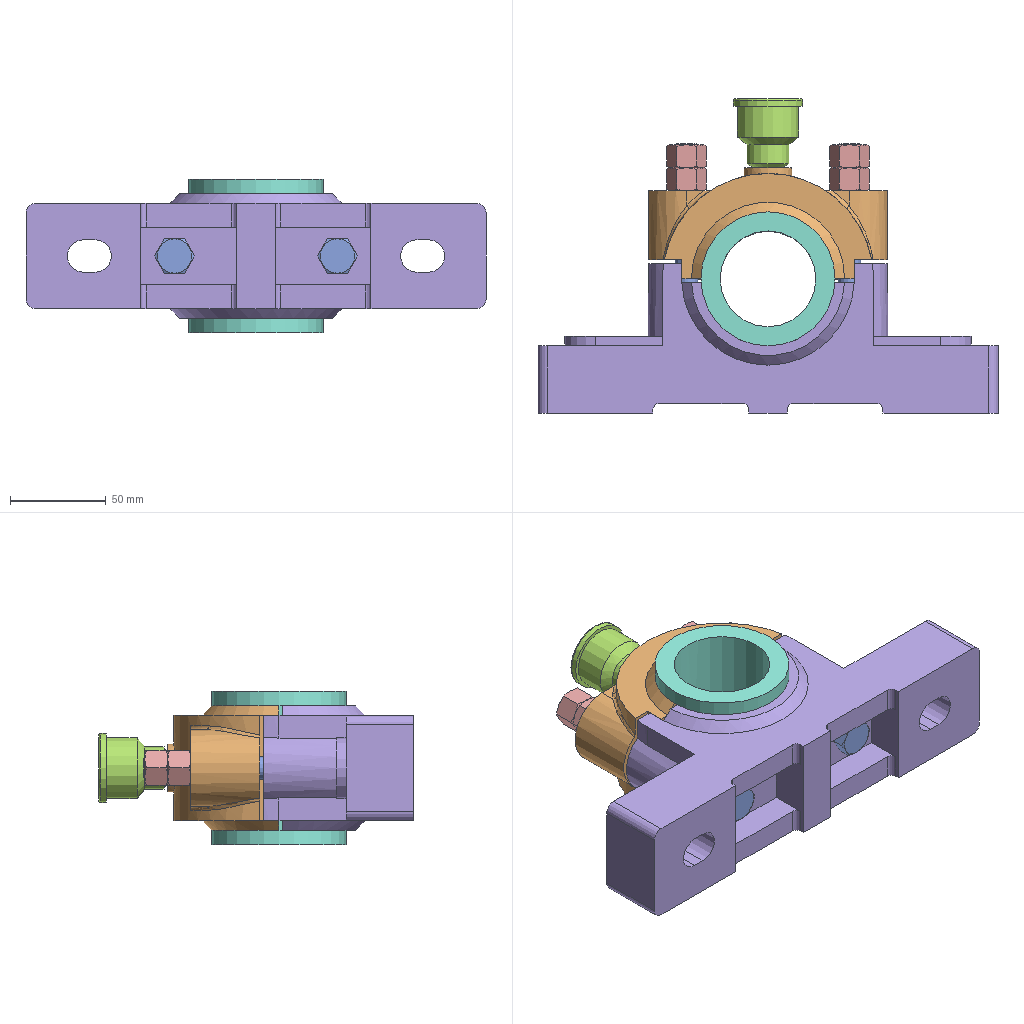Assembly | NX | 7 different items | 11 placed | box 240 x 164 x 80 mm
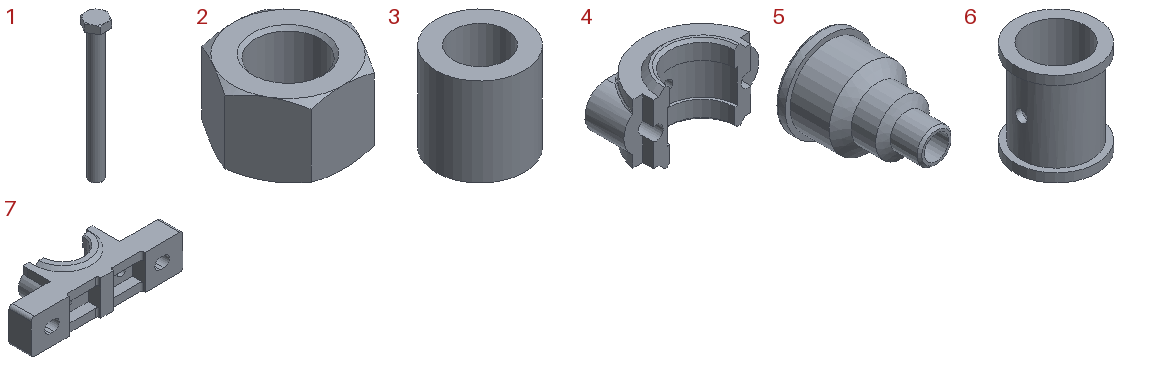Parts list (item | quantity | size | volume | features):
1 | x2 | 20.785 x 18 x 127.5 mm | 15029 mm3 | features SKETCH 4, EXTRUDE 3, META 3, DATUM_CSYS 2, BLEND 1, CHAMFER 1, DATUM_PLANE 1, LINE 1, SWP104 1, SYMBOLIC_THREAD 1, THREADS 1
2 | x4 | 20.785 x 18 x 12 mm | 2248 mm3 | features META 3, SKETCH 3, DATUM_CSYS 2, EXTRUDE 2, SWP104 2, CHAMFER 1, LINE 1, SYMBOLIC_THREAD 1, THREADS 1
3 | x1 | 10 x 10 x 10 mm | 502.655 mm3 | features DATUM_CSYS 1, EXTRUDE 1
4 | x1 | 125 x 58 x 65 mm | 196230 mm3 | features CHAMFER 4, HOLE PACKAGE 4, CYLINDER 3, DATUM_CSYS 3, EXTRUDE 3, SIMPLE HOLE 3, EXTRACT_STRING 2, SKETCH 2, ABSOLUTE_DATUM_PLANE 1, BLEND 1, BOSS 1, CBORE_HOLE 1, Instance Feature 1, Mirror Feature 1
5 | x1 | 36 x 48 x 36 mm | 9367 mm3 | features DATUM_CSYS 2, ABSOLUTE_DATUM_PLANE 1, BLEND 1, CHAMFER 1, SHELL 1, SKETCH 1, SWP104 1
6 | x1 | 70 x 70 x 80 mm | 84036 mm3 | features CYLINDER 5, DATUM_CSYS 1
7 | x1 | 240 x 78 x 65 mm | 522109 mm3 | features DATUM_CSYS 7, EXTRUDE 6, SKETCH 6, CYLINDER 3, SIMPLE HOLE 3, ABSOLUTE_DATUM_PLANE 2, CHAMFER 2, HOLE PACKAGE 2, BLEND 1
Mates (type | each side: item.copy, entity, surface, feature):
Touch | 7.1 face cylinder Ø60 Hole(11) | 4.1 face cylinder Ø60 Hole(7)
Touch | 7.1 face cylinder Ø13 Hole(10) | 4.1 face cylinder Ø13 Hole(5)
Touch | 6.1 face cylinder Cylinder(5) | 4.1 face cylinder Ø10 Counterbored Hole(12)
Touch | 6.1 face cylinder Cylinder(4) | 7.1 face cylinder Ø60 Hole(11)
Concentric | 3.1 edge | 4.1 edge
Concentric | 5.1 edge | 4.1 edge
Touch | 1.1 face cylinder Extrude(9) | 4.1 face cylinder Ø13 Hole(5)
Distance | 1.1 face plane Extrude(6) | 7.1 face plane Extrude(18)
Fix | assembly component
Bond | 1.1 component | assembly component | 2 times
LinearPattern | assembly axis | assembly csys | assembly csys
Concentric | 2.1 arc | 4.1 edge
Concentric | 2.1 arc | 2.1 edge